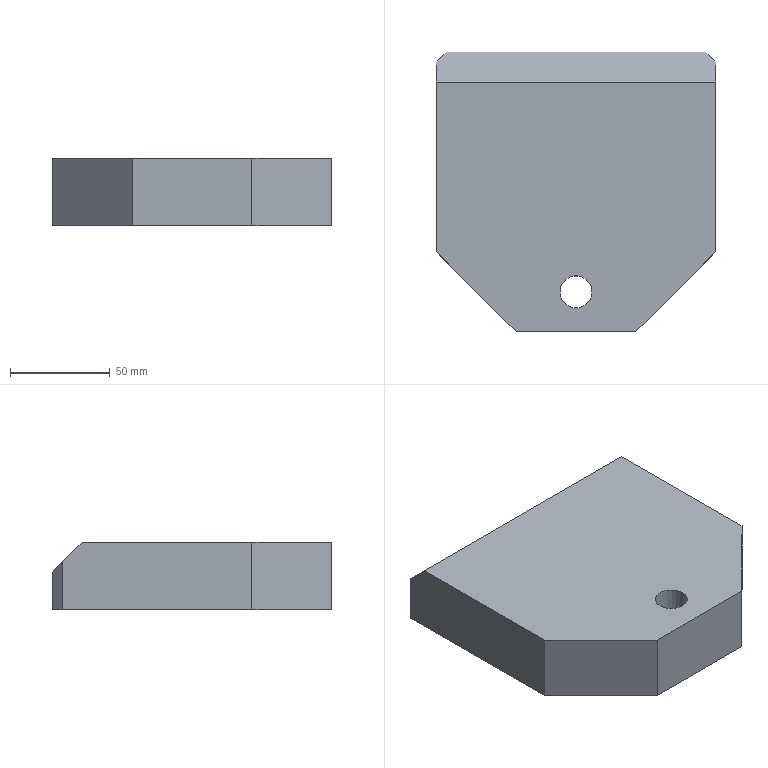Part | SolidWorks | features Chamfer 3, Extrusion 1, ICE 1 | 1 solid | 13 faces | box 140 x 140 x 34 mm | volume 588897 mm3 | plane 11 | cylinder 2 | commonest cylinder face diameters 16 x2
STEP:
#1=CARTESIAN_POINT('',(-8.,-50.,0.));
#2=VERTEX_POINT('',#1);
#3=CARTESIAN_POINT('',(8.,-50.,0.));
#4=VERTEX_POINT('',#3);
#5=CARTESIAN_POINT('',(0.,-50.,0.));
#6=DIRECTION('',(0.,0.,1.));
#7=DIRECTION('',(1.,0.,0.));
#8=AXIS2_PLACEMENT_3D('',#5,#6,#7);
#9=CIRCLE('',#8,8.);
#10=EDGE_CURVE('',#2,#4,#9,.T.);
#11=ORIENTED_EDGE('',*,*,#10,.F.);
#12=CARTESIAN_POINT('',(-8.,-50.,34.));
#13=VERTEX_POINT('',#12);
#14=CARTESIAN_POINT('',(-8.,-50.,0.));
#15=DIRECTION('',(0.,0.,1.));
#16=VECTOR('',#15,1000.);
#17=LINE('',#14,#16);
#18=EDGE_CURVE('',#2,#13,#17,.T.);
#19=ORIENTED_EDGE('',*,*,#18,.T.);
#20=CARTESIAN_POINT('',(8.,-50.,34.));
#21=VERTEX_POINT('',#20);
#22=CARTESIAN_POINT('',(0.,-50.,34.));
#23=DIRECTION('',(0.,0.,1.));
#24=DIRECTION('',(1.,0.,0.));
#25=AXIS2_PLACEMENT_3D('',#22,#23,#24);
#26=CIRCLE('',#25,8.);
#27=EDGE_CURVE('',#13,#21,#26,.T.);
#28=ORIENTED_EDGE('',*,*,#27,.T.);
#29=CARTESIAN_POINT('',(8.,-50.,0.));
#30=DIRECTION('',(0.,0.,1.));
#31=VECTOR('',#30,1000.);
#32=LINE('',#29,#31);
#33=EDGE_CURVE('',#4,#21,#32,.T.);
#34=ORIENTED_EDGE('',*,*,#33,.F.);
#35=EDGE_LOOP('',(#11,#19,#28,#34));
#36=FACE_OUTER_BOUND('',#35,.T.);
#37=CARTESIAN_POINT('',(0.,-50.,0.));
#38=DIRECTION('',(0.,0.,1.));
#39=DIRECTION('',(1.,0.,0.));
#40=AXIS2_PLACEMENT_3D('',#37,#38,#39);
#41=CYLINDRICAL_SURFACE('',#40,8.);
#42=ADVANCED_FACE('',(#36),#41,.F.);
#43=CARTESIAN_POINT('',(-70.,65.,0.));
#44=VERTEX_POINT('',#43);
#45=CARTESIAN_POINT('',(-70.,-30.,0.));
#46=VERTEX_POINT('',#45);
#47=CARTESIAN_POINT('',(-70.,-70.,0.));
#48=DIRECTION('',(0.,-1.,0.));
#49=VECTOR('',#48,1000.);
#50=LINE('',#47,#49);
#51=EDGE_CURVE('',#44,#46,#50,.T.);
#52=ORIENTED_EDGE('',*,*,#51,.T.);
#53=CARTESIAN_POINT('',(-70.,-30.,34.));
#54=VERTEX_POINT('',#53);
#55=CARTESIAN_POINT('',(-70.,-30.,34.));
#56=DIRECTION('',(0.,0.,1.));
#57=VECTOR('',#56,1000.);
#58=LINE('',#55,#57);
#59=EDGE_CURVE('',#46,#54,#58,.T.);
#60=ORIENTED_EDGE('',*,*,#59,.T.);
#61=CARTESIAN_POINT('',(-70.,55.,34.));
#62=VERTEX_POINT('',#61);
#63=CARTESIAN_POINT('',(-70.,-70.,34.));
#64=DIRECTION('',(0.,-1.,0.));
#65=VECTOR('',#64,1000.);
#66=LINE('',#63,#65);
#67=EDGE_CURVE('',#62,#54,#66,.T.);
#68=ORIENTED_EDGE('',*,*,#67,.F.);
#69=CARTESIAN_POINT('',(-70.,65.,24.));
#70=VERTEX_POINT('',#69);
#71=CARTESIAN_POINT('',(-70.,55.,34.));
#72=DIRECTION('',(0.,0.7071,-0.7071));
#73=VECTOR('',#72,1000.);
#74=LINE('',#71,#73);
#75=EDGE_CURVE('',#62,#70,#74,.T.);
#76=ORIENTED_EDGE('',*,*,#75,.T.);
#77=CARTESIAN_POINT('',(-70.,65.,34.));
#78=DIRECTION('',(0.,0.,-1.));
#79=VECTOR('',#78,1000.);
#80=LINE('',#77,#79);
#81=EDGE_CURVE('',#70,#44,#80,.T.);
#82=ORIENTED_EDGE('',*,*,#81,.T.);
#83=EDGE_LOOP('',(#52,#60,#68,#76,#82));
#84=FACE_OUTER_BOUND('',#83,.T.);
#85=CARTESIAN_POINT('',(-70.,-70.,34.));
#86=DIRECTION('',(1.,0.,0.));
#87=DIRECTION('',(0.,0.,-1.));
#88=AXIS2_PLACEMENT_3D('',#85,#86,#87);
#89=PLANE('',#88);
#90=ADVANCED_FACE('',(#84),#89,.F.);
#91=CARTESIAN_POINT('',(-30.,-70.,0.));
#92=VERTEX_POINT('',#91);
#93=CARTESIAN_POINT('',(30.,-70.,0.));
#94=VERTEX_POINT('',#93);
#95=CARTESIAN_POINT('',(70.,-70.,0.));
#96=DIRECTION('',(1.,0.,0.));
#97=VECTOR('',#96,1000.);
#98=LINE('',#95,#97);
#99=EDGE_CURVE('',#92,#94,#98,.T.);
#100=ORIENTED_EDGE('',*,*,#99,.T.);
#101=CARTESIAN_POINT('',(30.,-70.,34.));
#102=VERTEX_POINT('',#101);
#103=CARTESIAN_POINT('',(30.,-70.,34.));
#104=DIRECTION('',(0.,0.,1.));
#105=VECTOR('',#104,1000.);
#106=LINE('',#103,#105);
#107=EDGE_CURVE('',#94,#102,#106,.T.);
#108=ORIENTED_EDGE('',*,*,#107,.T.);
#109=CARTESIAN_POINT('',(-30.,-70.,34.));
#110=VERTEX_POINT('',#109);
#111=CARTESIAN_POINT('',(70.,-70.,34.));
#112=DIRECTION('',(1.,0.,0.));
#113=VECTOR('',#112,1000.);
#114=LINE('',#111,#113);
#115=EDGE_CURVE('',#110,#102,#114,.T.);
#116=ORIENTED_EDGE('',*,*,#115,.F.);
#117=CARTESIAN_POINT('',(-30.,-70.,34.));
#118=DIRECTION('',(0.,0.,-1.));
#119=VECTOR('',#118,1000.);
#120=LINE('',#117,#119);
#121=EDGE_CURVE('',#110,#92,#120,.T.);
#122=ORIENTED_EDGE('',*,*,#121,.T.);
#123=EDGE_LOOP('',(#100,#108,#116,#122));
#124=FACE_OUTER_BOUND('',#123,.T.);
#125=CARTESIAN_POINT('',(70.,-70.,34.));
#126=DIRECTION('',(0.,1.,0.));
#127=DIRECTION('',(-1.,0.,0.));
#128=AXIS2_PLACEMENT_3D('',#125,#126,#127);
#129=PLANE('',#128);
#130=ADVANCED_FACE('',(#124),#129,.F.);
#131=CARTESIAN_POINT('',(70.,-30.,34.));
#132=VERTEX_POINT('',#131);
#133=CARTESIAN_POINT('',(70.,55.,34.));
#134=VERTEX_POINT('',#133);
#135=CARTESIAN_POINT('',(70.,-70.,34.));
#136=DIRECTION('',(0.,1.,0.));
#137=VECTOR('',#136,1000.);
#138=LINE('',#135,#137);
#139=EDGE_CURVE('',#132,#134,#138,.T.);
#140=ORIENTED_EDGE('',*,*,#139,.F.);
#141=CARTESIAN_POINT('',(70.,-30.,0.));
#142=VERTEX_POINT('',#141);
#143=CARTESIAN_POINT('',(70.,-30.,34.));
#144=DIRECTION('',(0.,0.,-1.));
#145=VECTOR('',#144,1000.);
#146=LINE('',#143,#145);
#147=EDGE_CURVE('',#132,#142,#146,.T.);
#148=ORIENTED_EDGE('',*,*,#147,.T.);
#149=CARTESIAN_POINT('',(70.,65.,0.));
#150=VERTEX_POINT('',#149);
#151=CARTESIAN_POINT('',(70.,-70.,0.));
#152=DIRECTION('',(0.,1.,0.));
#153=VECTOR('',#152,1000.);
#154=LINE('',#151,#153);
#155=EDGE_CURVE('',#142,#150,#154,.T.);
#156=ORIENTED_EDGE('',*,*,#155,.T.);
#157=CARTESIAN_POINT('',(70.,65.,24.));
#158=VERTEX_POINT('',#157);
#159=CARTESIAN_POINT('',(70.,65.,34.));
#160=DIRECTION('',(0.,0.,1.));
#161=VECTOR('',#160,1000.);
#162=LINE('',#159,#161);
#163=EDGE_CURVE('',#150,#158,#162,.T.);
#164=ORIENTED_EDGE('',*,*,#163,.T.);
#165=CARTESIAN_POINT('',(70.,55.,34.));
#166=DIRECTION('',(0.,-0.7071,0.7071));
#167=VECTOR('',#166,1000.);
#168=LINE('',#165,#167);
#169=EDGE_CURVE('',#158,#134,#168,.T.);
#170=ORIENTED_EDGE('',*,*,#169,.T.);
#171=EDGE_LOOP('',(#140,#148,#156,#164,#170));
#172=FACE_OUTER_BOUND('',#171,.T.);
#173=CARTESIAN_POINT('',(70.,-70.,34.));
#174=DIRECTION('',(-1.,0.,0.));
#175=DIRECTION('',(0.,0.,1.));
#176=AXIS2_PLACEMENT_3D('',#173,#174,#175);
#177=PLANE('',#176);
#178=ADVANCED_FACE('',(#172),#177,.F.);
#179=CARTESIAN_POINT('',(-65.,70.,0.));
#180=VERTEX_POINT('',#179);
#181=CARTESIAN_POINT('',(-65.,70.,19.));
#182=VERTEX_POINT('',#181);
#183=CARTESIAN_POINT('',(-65.,70.,34.));
#184=DIRECTION('',(0.,0.,1.));
#185=VECTOR('',#184,1000.);
#186=LINE('',#183,#185);
#187=EDGE_CURVE('',#180,#182,#186,.T.);
#188=ORIENTED_EDGE('',*,*,#187,.T.);
#189=CARTESIAN_POINT('',(65.,70.,19.));
#190=VERTEX_POINT('',#189);
#191=CARTESIAN_POINT('',(65.,70.,19.));
#192=DIRECTION('',(1.,0.,0.));
#193=VECTOR('',#192,1000.);
#194=LINE('',#191,#193);
#195=EDGE_CURVE('',#182,#190,#194,.T.);
#196=ORIENTED_EDGE('',*,*,#195,.T.);
#197=CARTESIAN_POINT('',(65.,70.,0.));
#198=VERTEX_POINT('',#197);
#199=CARTESIAN_POINT('',(65.,70.,34.));
#200=DIRECTION('',(0.,0.,-1.));
#201=VECTOR('',#200,1000.);
#202=LINE('',#199,#201);
#203=EDGE_CURVE('',#190,#198,#202,.T.);
#204=ORIENTED_EDGE('',*,*,#203,.T.);
#205=CARTESIAN_POINT('',(70.,70.,0.));
#206=DIRECTION('',(-1.,0.,0.));
#207=VECTOR('',#206,1000.);
#208=LINE('',#205,#207);
#209=EDGE_CURVE('',#198,#180,#208,.T.);
#210=ORIENTED_EDGE('',*,*,#209,.T.);
#211=EDGE_LOOP('',(#188,#196,#204,#210));
#212=FACE_OUTER_BOUND('',#211,.T.);
#213=CARTESIAN_POINT('',(70.,70.,34.));
#214=DIRECTION('',(0.,-1.,0.));
#215=DIRECTION('',(1.,0.,0.));
#216=AXIS2_PLACEMENT_3D('',#213,#214,#215);
#217=PLANE('',#216);
#218=ADVANCED_FACE('',(#212),#217,.F.);
#219=CARTESIAN_POINT('',(0.,-50.,34.));
#220=DIRECTION('',(0.,0.,1.));
#221=DIRECTION('',(1.,0.,0.));
#222=AXIS2_PLACEMENT_3D('',#219,#220,#221);
#223=CIRCLE('',#222,8.);
#224=EDGE_CURVE('',#21,#13,#223,.T.);
#225=ORIENTED_EDGE('',*,*,#224,.F.);
#226=ORIENTED_EDGE('',*,*,#27,.F.);
#227=EDGE_LOOP('',(#225,#226));
#228=FACE_BOUND('',#227,.T.);
#229=ORIENTED_EDGE('',*,*,#115,.T.);
#230=CARTESIAN_POINT('',(50.,-50.,34.));
#231=DIRECTION('',(0.7071,0.7071,0.));
#232=VECTOR('',#231,1000.);
#233=LINE('',#230,#232);
#234=EDGE_CURVE('',#102,#132,#233,.T.);
#235=ORIENTED_EDGE('',*,*,#234,.T.);
#236=ORIENTED_EDGE('',*,*,#139,.T.);
#237=CARTESIAN_POINT('',(-65.,55.,34.));
#238=DIRECTION('',(-1.,0.,0.));
#239=VECTOR('',#238,1000.);
#240=LINE('',#237,#239);
#241=EDGE_CURVE('',#134,#62,#240,.T.);
#242=ORIENTED_EDGE('',*,*,#241,.T.);
#243=ORIENTED_EDGE('',*,*,#67,.T.);
#244=CARTESIAN_POINT('',(-50.,-50.,34.));
#245=DIRECTION('',(0.7071,-0.7071,0.));
#246=VECTOR('',#245,1000.);
#247=LINE('',#244,#246);
#248=EDGE_CURVE('',#54,#110,#247,.T.);
#249=ORIENTED_EDGE('',*,*,#248,.T.);
#250=EDGE_LOOP('',(#229,#235,#236,#242,#243,#249));
#251=FACE_OUTER_BOUND('',#250,.T.);
#252=CARTESIAN_POINT('',(0.,0.,34.));
#253=DIRECTION('',(0.,0.,1.));
#254=DIRECTION('',(1.,0.,0.));
#255=AXIS2_PLACEMENT_3D('',#252,#253,#254);
#256=PLANE('',#255);
#257=ADVANCED_FACE('',(#228,#251),#256,.T.);
#258=CARTESIAN_POINT('',(0.,-50.,0.));
#259=DIRECTION('',(0.,0.,1.));
#260=DIRECTION('',(1.,0.,0.));
#261=AXIS2_PLACEMENT_3D('',#258,#259,#260);
#262=CIRCLE('',#261,8.);
#263=EDGE_CURVE('',#4,#2,#262,.T.);
#264=ORIENTED_EDGE('',*,*,#263,.T.);
#265=ORIENTED_EDGE('',*,*,#10,.T.);
#266=EDGE_LOOP('',(#264,#265));
#267=FACE_BOUND('',#266,.T.);
#268=ORIENTED_EDGE('',*,*,#155,.F.);
#269=CARTESIAN_POINT('',(70.,-30.,0.));
#270=DIRECTION('',(-0.7071,-0.7071,0.));
#271=VECTOR('',#270,1000.);
#272=LINE('',#269,#271);
#273=EDGE_CURVE('',#142,#94,#272,.T.);
#274=ORIENTED_EDGE('',*,*,#273,.T.);
#275=ORIENTED_EDGE('',*,*,#99,.F.);
#276=CARTESIAN_POINT('',(-30.,-70.,0.));
#277=DIRECTION('',(-0.7071,0.7071,0.));
#278=VECTOR('',#277,1000.);
#279=LINE('',#276,#278);
#280=EDGE_CURVE('',#92,#46,#279,.T.);
#281=ORIENTED_EDGE('',*,*,#280,.T.);
#282=ORIENTED_EDGE('',*,*,#51,.F.);
#283=CARTESIAN_POINT('',(-70.,65.,0.));
#284=DIRECTION('',(0.7071,0.7071,0.));
#285=VECTOR('',#284,1000.);
#286=LINE('',#283,#285);
#287=EDGE_CURVE('',#44,#180,#286,.T.);
#288=ORIENTED_EDGE('',*,*,#287,.T.);
#289=ORIENTED_EDGE('',*,*,#209,.F.);
#290=CARTESIAN_POINT('',(65.,70.,0.));
#291=DIRECTION('',(0.7071,-0.7071,0.));
#292=VECTOR('',#291,1000.);
#293=LINE('',#290,#292);
#294=EDGE_CURVE('',#198,#150,#293,.T.);
#295=ORIENTED_EDGE('',*,*,#294,.T.);
#296=EDGE_LOOP('',(#268,#274,#275,#281,#282,#288,#289,#295));
#297=FACE_OUTER_BOUND('',#296,.T.);
#298=CARTESIAN_POINT('',(0.,0.,0.));
#299=DIRECTION('',(0.,0.,1.));
#300=DIRECTION('',(1.,0.,0.));
#301=AXIS2_PLACEMENT_3D('',#298,#299,#300);
#302=PLANE('',#301);
#303=ADVANCED_FACE('',(#267,#297),#302,.F.);
#304=ORIENTED_EDGE('',*,*,#18,.F.);
#305=ORIENTED_EDGE('',*,*,#263,.F.);
#306=ORIENTED_EDGE('',*,*,#33,.T.);
#307=ORIENTED_EDGE('',*,*,#224,.T.);
#308=EDGE_LOOP('',(#304,#305,#306,#307));
#309=FACE_OUTER_BOUND('',#308,.T.);
#310=CARTESIAN_POINT('',(0.,-50.,0.));
#311=DIRECTION('',(0.,0.,1.));
#312=DIRECTION('',(1.,0.,0.));
#313=AXIS2_PLACEMENT_3D('',#310,#311,#312);
#314=CYLINDRICAL_SURFACE('',#313,8.);
#315=ADVANCED_FACE('',(#309),#314,.F.);
#316=ORIENTED_EDGE('',*,*,#203,.F.);
#317=CARTESIAN_POINT('',(70.,65.,24.));
#318=DIRECTION('',(0.5774,-0.5774,0.5774));
#319=VECTOR('',#318,1000.);
#320=LINE('',#317,#319);
#321=EDGE_CURVE('',#190,#158,#320,.T.);
#322=ORIENTED_EDGE('',*,*,#321,.T.);
#323=ORIENTED_EDGE('',*,*,#163,.F.);
#324=ORIENTED_EDGE('',*,*,#294,.F.);
#325=EDGE_LOOP('',(#316,#322,#323,#324));
#326=FACE_OUTER_BOUND('',#325,.T.);
#327=CARTESIAN_POINT('',(65.,70.,34.));
#328=DIRECTION('',(-0.7071,-0.7071,0.));
#329=DIRECTION('',(0.,0.,-1.));
#330=AXIS2_PLACEMENT_3D('',#327,#328,#329);
#331=PLANE('',#330);
#332=ADVANCED_FACE('',(#326),#331,.F.);
#333=ORIENTED_EDGE('',*,*,#81,.F.);
#334=CARTESIAN_POINT('',(-73.333,61.667,27.333));
#335=DIRECTION('',(0.5774,0.5774,-0.5774));
#336=VECTOR('',#335,1000.);
#337=LINE('',#334,#336);
#338=EDGE_CURVE('',#70,#182,#337,.T.);
#339=ORIENTED_EDGE('',*,*,#338,.T.);
#340=ORIENTED_EDGE('',*,*,#187,.F.);
#341=ORIENTED_EDGE('',*,*,#287,.F.);
#342=EDGE_LOOP('',(#333,#339,#340,#341));
#343=FACE_OUTER_BOUND('',#342,.T.);
#344=CARTESIAN_POINT('',(-70.,65.,34.));
#345=DIRECTION('',(0.7071,-0.7071,0.));
#346=DIRECTION('',(0.,0.,-1.));
#347=AXIS2_PLACEMENT_3D('',#344,#345,#346);
#348=PLANE('',#347);
#349=ADVANCED_FACE('',(#343),#348,.F.);
#350=ORIENTED_EDGE('',*,*,#321,.F.);
#351=ORIENTED_EDGE('',*,*,#195,.F.);
#352=ORIENTED_EDGE('',*,*,#338,.F.);
#353=ORIENTED_EDGE('',*,*,#75,.F.);
#354=ORIENTED_EDGE('',*,*,#241,.F.);
#355=ORIENTED_EDGE('',*,*,#169,.F.);
#356=EDGE_LOOP('',(#350,#351,#352,#353,#354,#355));
#357=FACE_OUTER_BOUND('',#356,.T.);
#358=CARTESIAN_POINT('',(0.,55.,34.));
#359=DIRECTION('',(0.,0.7071,0.7071));
#360=DIRECTION('',(1.,0.,0.));
#361=AXIS2_PLACEMENT_3D('',#358,#359,#360);
#362=PLANE('',#361);
#363=ADVANCED_FACE('',(#357),#362,.T.);
#364=ORIENTED_EDGE('',*,*,#234,.F.);
#365=ORIENTED_EDGE('',*,*,#107,.F.);
#366=ORIENTED_EDGE('',*,*,#273,.F.);
#367=ORIENTED_EDGE('',*,*,#147,.F.);
#368=EDGE_LOOP('',(#364,#365,#366,#367));
#369=FACE_OUTER_BOUND('',#368,.T.);
#370=CARTESIAN_POINT('',(70.,-30.,34.));
#371=DIRECTION('',(-0.7071,0.7071,0.));
#372=DIRECTION('',(0.,0.,-1.));
#373=AXIS2_PLACEMENT_3D('',#370,#371,#372);
#374=PLANE('',#373);
#375=ADVANCED_FACE('',(#369),#374,.F.);
#376=ORIENTED_EDGE('',*,*,#248,.F.);
#377=ORIENTED_EDGE('',*,*,#59,.F.);
#378=ORIENTED_EDGE('',*,*,#280,.F.);
#379=ORIENTED_EDGE('',*,*,#121,.F.);
#380=EDGE_LOOP('',(#376,#377,#378,#379));
#381=FACE_OUTER_BOUND('',#380,.T.);
#382=CARTESIAN_POINT('',(-30.,-70.,34.));
#383=DIRECTION('',(0.7071,0.7071,0.));
#384=DIRECTION('',(0.,0.,-1.));
#385=AXIS2_PLACEMENT_3D('',#382,#383,#384);
#386=PLANE('',#385);
#387=ADVANCED_FACE('',(#381),#386,.F.);
#388=CLOSED_SHELL('',(#42,#90,#130,#178,#218,#257,#303,#315,#332,#349,#363,#375,#387));
#389=MANIFOLD_SOLID_BREP('',#388);
#390=CARTESIAN_POINT('',(0.,0.,0.));
#391=DIRECTION('',(0.,0.,1.));
#392=DIRECTION('',(1.,0.,0.));
#393=AXIS2_PLACEMENT_3D('',#390,#391,#392);
#394=(LENGTH_UNIT()NAMED_UNIT(*)SI_UNIT(.MILLI.,.METRE.));
#395=UNCERTAINTY_MEASURE_WITH_UNIT(LENGTH_MEASURE(0.00001),#394,'','');
#396=(NAMED_UNIT(*)PLANE_ANGLE_UNIT()SI_UNIT($,.RADIAN.));
#397=(NAMED_UNIT(*)SI_UNIT($,.STERADIAN.)SOLID_ANGLE_UNIT());
#398=(GEOMETRIC_REPRESENTATION_CONTEXT(3)GLOBAL_UNCERTAINTY_ASSIGNED_CONTEXT((#395))GLOBAL_UNIT_ASSIGNED_CONTEXT((#394,#396,#397))REPRESENTATION_CONTEXT('',''));
#399=ADVANCED_BREP_SHAPE_REPRESENTATION('',(#389,#393),#398);